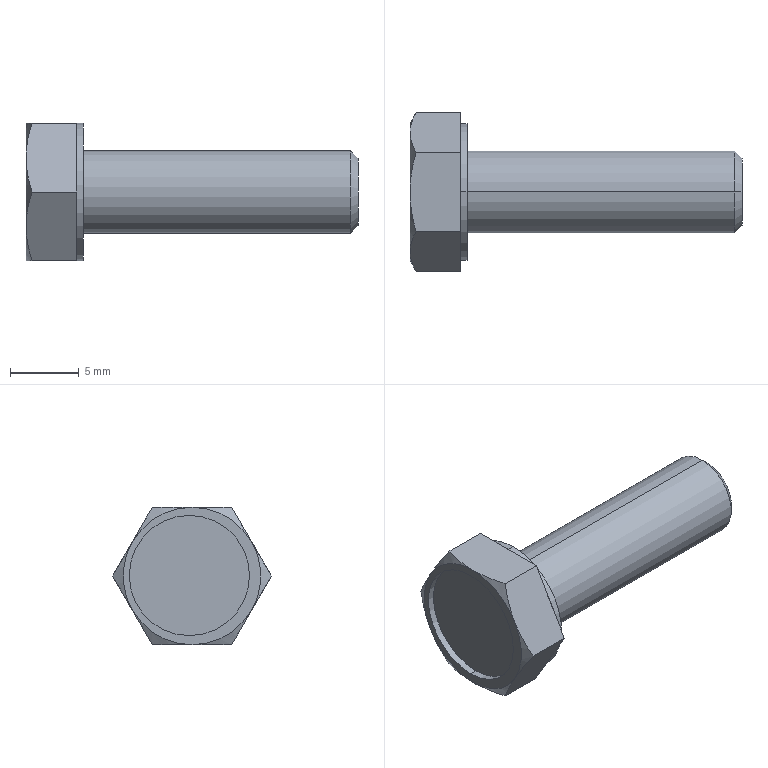Part | STEP file | formed hex screw_am_B18.2.3.2M - Formed hex screw, M6 x 1.0 x 20 --20WN | 1 solid | 30 faces | box 24.15 x 11.547 x 10 mm | volume 885.854 mm3 | plane 16 | cone 8 | cylinder 6 | commonest cylinder face diameters 6 x2 8.75 x2 10 x2